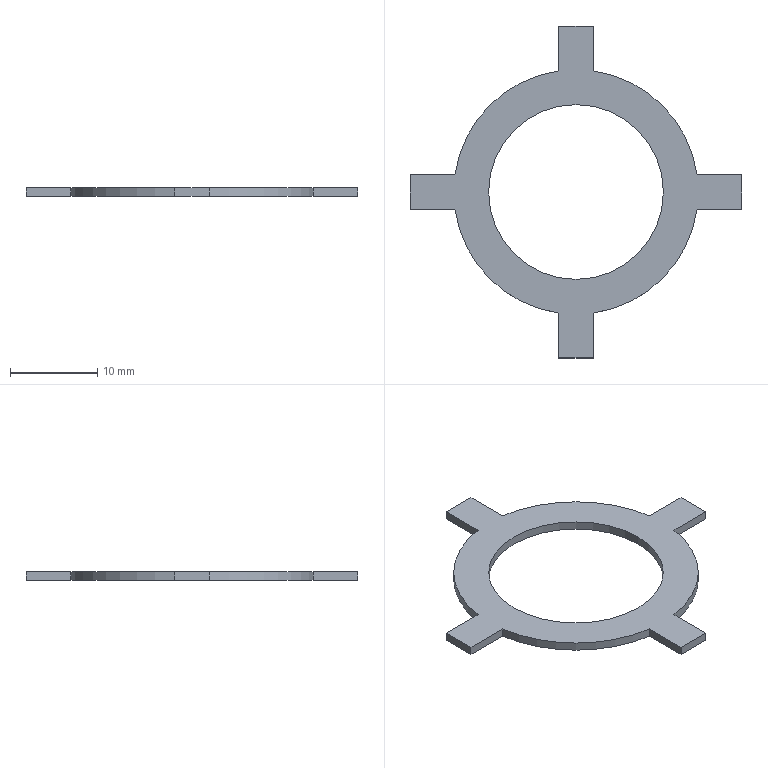Part | STEP file | ZDDQ-M20 | 1 solid | 20 faces | box 38 x 38 x 1 mm | volume 382.357 mm3 | plane 14 | cylinder 6 | commonest cylinder face diameters 28 x4 20 x2
STEP:
#1=CARTESIAN_POINT('',(-19.,2.,0.));
#2=VERTEX_POINT('',#1);
#3=CARTESIAN_POINT('',(-19.,-2.,0.));
#4=VERTEX_POINT('',#3);
#5=CARTESIAN_POINT('',(-19.,0.,0.));
#6=DIRECTION('',(0.,1.,0.));
#7=VECTOR('',#6,1.);
#8=LINE('',#5,#7);
#9=EDGE_CURVE('',#2,#4,#8,.F.);
#10=ORIENTED_EDGE('',*,*,#9,.T.);
#11=CARTESIAN_POINT('',(-19.,-2.,1.));
#12=VERTEX_POINT('',#11);
#13=CARTESIAN_POINT('',(-19.,-2.,0.5));
#14=DIRECTION('',(0.,0.,-1.));
#15=VECTOR('',#14,1.);
#16=LINE('',#13,#15);
#17=EDGE_CURVE('',#12,#4,#16,.T.);
#18=ORIENTED_EDGE('',*,*,#17,.F.);
#19=CARTESIAN_POINT('',(-19.,2.,1.));
#20=VERTEX_POINT('',#19);
#21=CARTESIAN_POINT('',(-19.,0.,1.));
#22=DIRECTION('',(0.,1.,0.));
#23=VECTOR('',#22,1.);
#24=LINE('',#21,#23);
#25=EDGE_CURVE('',#20,#12,#24,.F.);
#26=ORIENTED_EDGE('',*,*,#25,.F.);
#27=CARTESIAN_POINT('',(-19.,2.,0.5));
#28=DIRECTION('',(0.,0.,-1.));
#29=VECTOR('',#28,1.);
#30=LINE('',#27,#29);
#31=EDGE_CURVE('',#20,#2,#30,.T.);
#32=ORIENTED_EDGE('',*,*,#31,.T.);
#33=EDGE_LOOP('',(#10,#18,#26,#32));
#34=FACE_OUTER_BOUND('',#33,.T.);
#35=CARTESIAN_POINT('',(-19.,-2.,1.));
#36=DIRECTION('',(-1.,0.,0.));
#37=DIRECTION('',(0.,1.,0.));
#38=AXIS2_PLACEMENT_3D('',#35,#36,#37);
#39=PLANE('',#38);
#40=ADVANCED_FACE('',(#34),#39,.T.);
#41=CARTESIAN_POINT('',(-13.856,-2.,0.));
#42=VERTEX_POINT('',#41);
#43=CARTESIAN_POINT('',(-13.856,-2.,1.));
#44=VERTEX_POINT('',#43);
#45=CARTESIAN_POINT('',(-13.856,-2.,0.5));
#46=DIRECTION('',(0.,0.,1.));
#47=VECTOR('',#46,1.);
#48=LINE('',#45,#47);
#49=EDGE_CURVE('',#42,#44,#48,.T.);
#50=ORIENTED_EDGE('',*,*,#49,.T.);
#51=CARTESIAN_POINT('',(-16.428,-2.,1.));
#52=DIRECTION('',(1.,0.,0.));
#53=VECTOR('',#52,1.);
#54=LINE('',#51,#53);
#55=EDGE_CURVE('',#12,#44,#54,.T.);
#56=ORIENTED_EDGE('',*,*,#55,.F.);
#57=ORIENTED_EDGE('',*,*,#17,.T.);
#58=CARTESIAN_POINT('',(-16.428,-2.,0.));
#59=DIRECTION('',(1.,0.,0.));
#60=VECTOR('',#59,1.);
#61=LINE('',#58,#60);
#62=EDGE_CURVE('',#4,#42,#61,.T.);
#63=ORIENTED_EDGE('',*,*,#62,.T.);
#64=EDGE_LOOP('',(#50,#56,#57,#63));
#65=FACE_OUTER_BOUND('',#64,.T.);
#66=CARTESIAN_POINT('',(11.858,-2.,1.));
#67=DIRECTION('',(0.,1.,0.));
#68=DIRECTION('',(1.,0.,0.));
#69=AXIS2_PLACEMENT_3D('',#66,#67,#68);
#70=PLANE('',#69);
#71=ADVANCED_FACE('',(#65),#70,.F.);
#72=CARTESIAN_POINT('',(-13.856,2.,0.));
#73=VERTEX_POINT('',#72);
#74=CARTESIAN_POINT('',(-13.856,2.,1.));
#75=VERTEX_POINT('',#74);
#76=CARTESIAN_POINT('',(-13.856,2.,0.5));
#77=DIRECTION('',(0.,0.,1.));
#78=VECTOR('',#77,1.);
#79=LINE('',#76,#78);
#80=EDGE_CURVE('',#73,#75,#79,.T.);
#81=ORIENTED_EDGE('',*,*,#80,.F.);
#82=CARTESIAN_POINT('',(-16.428,2.,0.));
#83=DIRECTION('',(-1.,0.,0.));
#84=VECTOR('',#83,1.);
#85=LINE('',#82,#84);
#86=EDGE_CURVE('',#73,#2,#85,.T.);
#87=ORIENTED_EDGE('',*,*,#86,.T.);
#88=ORIENTED_EDGE('',*,*,#31,.F.);
#89=CARTESIAN_POINT('',(-16.428,2.,1.));
#90=DIRECTION('',(-1.,0.,0.));
#91=VECTOR('',#90,1.);
#92=LINE('',#89,#91);
#93=EDGE_CURVE('',#75,#20,#92,.T.);
#94=ORIENTED_EDGE('',*,*,#93,.F.);
#95=EDGE_LOOP('',(#81,#87,#88,#94));
#96=FACE_OUTER_BOUND('',#95,.T.);
#97=CARTESIAN_POINT('',(19.,2.,1.));
#98=DIRECTION('',(0.,-1.,0.));
#99=DIRECTION('',(-1.,0.,0.));
#100=AXIS2_PLACEMENT_3D('',#97,#98,#99);
#101=PLANE('',#100);
#102=ADVANCED_FACE('',(#96),#101,.F.);
#103=CARTESIAN_POINT('',(-2.,-19.,0.));
#104=VERTEX_POINT('',#103);
#105=CARTESIAN_POINT('',(2.,-19.,0.));
#106=VERTEX_POINT('',#105);
#107=CARTESIAN_POINT('',(0.,-19.,0.));
#108=DIRECTION('',(-1.,0.,0.));
#109=VECTOR('',#108,1.);
#110=LINE('',#107,#109);
#111=EDGE_CURVE('',#104,#106,#110,.F.);
#112=ORIENTED_EDGE('',*,*,#111,.T.);
#113=CARTESIAN_POINT('',(2.,-19.,1.));
#114=VERTEX_POINT('',#113);
#115=CARTESIAN_POINT('',(2.,-19.,0.5));
#116=DIRECTION('',(0.,0.,-1.));
#117=VECTOR('',#116,1.);
#118=LINE('',#115,#117);
#119=EDGE_CURVE('',#114,#106,#118,.T.);
#120=ORIENTED_EDGE('',*,*,#119,.F.);
#121=CARTESIAN_POINT('',(-2.,-19.,1.));
#122=VERTEX_POINT('',#121);
#123=CARTESIAN_POINT('',(0.,-19.,1.));
#124=DIRECTION('',(-1.,0.,0.));
#125=VECTOR('',#124,1.);
#126=LINE('',#123,#125);
#127=EDGE_CURVE('',#122,#114,#126,.F.);
#128=ORIENTED_EDGE('',*,*,#127,.F.);
#129=CARTESIAN_POINT('',(-2.,-19.,0.5));
#130=DIRECTION('',(0.,0.,-1.));
#131=VECTOR('',#130,1.);
#132=LINE('',#129,#131);
#133=EDGE_CURVE('',#122,#104,#132,.T.);
#134=ORIENTED_EDGE('',*,*,#133,.T.);
#135=EDGE_LOOP('',(#112,#120,#128,#134));
#136=FACE_OUTER_BOUND('',#135,.T.);
#137=CARTESIAN_POINT('',(2.,-19.,1.));
#138=DIRECTION('',(0.,-1.,0.));
#139=DIRECTION('',(-1.,0.,0.));
#140=AXIS2_PLACEMENT_3D('',#137,#138,#139);
#141=PLANE('',#140);
#142=ADVANCED_FACE('',(#136),#141,.T.);
#143=CARTESIAN_POINT('',(2.,-13.856,0.));
#144=VERTEX_POINT('',#143);
#145=CARTESIAN_POINT('',(2.,-13.856,1.));
#146=VERTEX_POINT('',#145);
#147=CARTESIAN_POINT('',(2.,-13.856,0.5));
#148=DIRECTION('',(0.,0.,1.));
#149=VECTOR('',#148,1.);
#150=LINE('',#147,#149);
#151=EDGE_CURVE('',#144,#146,#150,.T.);
#152=ORIENTED_EDGE('',*,*,#151,.T.);
#153=CARTESIAN_POINT('',(2.,-16.428,1.));
#154=DIRECTION('',(0.,1.,0.));
#155=VECTOR('',#154,1.);
#156=LINE('',#153,#155);
#157=EDGE_CURVE('',#114,#146,#156,.T.);
#158=ORIENTED_EDGE('',*,*,#157,.F.);
#159=ORIENTED_EDGE('',*,*,#119,.T.);
#160=CARTESIAN_POINT('',(2.,-16.428,0.));
#161=DIRECTION('',(0.,1.,0.));
#162=VECTOR('',#161,1.);
#163=LINE('',#160,#162);
#164=EDGE_CURVE('',#106,#144,#163,.T.);
#165=ORIENTED_EDGE('',*,*,#164,.T.);
#166=EDGE_LOOP('',(#152,#158,#159,#165));
#167=FACE_OUTER_BOUND('',#166,.T.);
#168=CARTESIAN_POINT('',(2.,11.858,1.));
#169=DIRECTION('',(-1.,0.,0.));
#170=DIRECTION('',(0.,1.,0.));
#171=AXIS2_PLACEMENT_3D('',#168,#169,#170);
#172=PLANE('',#171);
#173=ADVANCED_FACE('',(#167),#172,.F.);
#174=CARTESIAN_POINT('',(-2.,-13.856,0.));
#175=VERTEX_POINT('',#174);
#176=CARTESIAN_POINT('',(-2.,-13.856,1.));
#177=VERTEX_POINT('',#176);
#178=CARTESIAN_POINT('',(-2.,-13.856,0.5));
#179=DIRECTION('',(0.,0.,1.));
#180=VECTOR('',#179,1.);
#181=LINE('',#178,#180);
#182=EDGE_CURVE('',#175,#177,#181,.T.);
#183=ORIENTED_EDGE('',*,*,#182,.F.);
#184=CARTESIAN_POINT('',(-2.,-16.428,0.));
#185=DIRECTION('',(0.,-1.,0.));
#186=VECTOR('',#185,1.);
#187=LINE('',#184,#186);
#188=EDGE_CURVE('',#175,#104,#187,.T.);
#189=ORIENTED_EDGE('',*,*,#188,.T.);
#190=ORIENTED_EDGE('',*,*,#133,.F.);
#191=CARTESIAN_POINT('',(-2.,-16.428,1.));
#192=DIRECTION('',(0.,-1.,0.));
#193=VECTOR('',#192,1.);
#194=LINE('',#191,#193);
#195=EDGE_CURVE('',#177,#122,#194,.T.);
#196=ORIENTED_EDGE('',*,*,#195,.F.);
#197=EDGE_LOOP('',(#183,#189,#190,#196));
#198=FACE_OUTER_BOUND('',#197,.T.);
#199=CARTESIAN_POINT('',(-2.,19.,1.));
#200=DIRECTION('',(1.,0.,0.));
#201=DIRECTION('',(0.,-1.,0.));
#202=AXIS2_PLACEMENT_3D('',#199,#200,#201);
#203=PLANE('',#202);
#204=ADVANCED_FACE('',(#198),#203,.F.);
#205=CARTESIAN_POINT('',(19.,-2.,0.));
#206=VERTEX_POINT('',#205);
#207=CARTESIAN_POINT('',(19.,2.,0.));
#208=VERTEX_POINT('',#207);
#209=CARTESIAN_POINT('',(19.,0.,0.));
#210=DIRECTION('',(0.,-1.,0.));
#211=VECTOR('',#210,1.);
#212=LINE('',#209,#211);
#213=EDGE_CURVE('',#206,#208,#212,.F.);
#214=ORIENTED_EDGE('',*,*,#213,.T.);
#215=CARTESIAN_POINT('',(19.,2.,1.));
#216=VERTEX_POINT('',#215);
#217=CARTESIAN_POINT('',(19.,2.,0.5));
#218=DIRECTION('',(0.,0.,-1.));
#219=VECTOR('',#218,1.);
#220=LINE('',#217,#219);
#221=EDGE_CURVE('',#216,#208,#220,.T.);
#222=ORIENTED_EDGE('',*,*,#221,.F.);
#223=CARTESIAN_POINT('',(19.,-2.,1.));
#224=VERTEX_POINT('',#223);
#225=CARTESIAN_POINT('',(19.,0.,1.));
#226=DIRECTION('',(0.,-1.,0.));
#227=VECTOR('',#226,1.);
#228=LINE('',#225,#227);
#229=EDGE_CURVE('',#224,#216,#228,.F.);
#230=ORIENTED_EDGE('',*,*,#229,.F.);
#231=CARTESIAN_POINT('',(19.,-2.,0.5));
#232=DIRECTION('',(0.,0.,-1.));
#233=VECTOR('',#232,1.);
#234=LINE('',#231,#233);
#235=EDGE_CURVE('',#224,#206,#234,.T.);
#236=ORIENTED_EDGE('',*,*,#235,.T.);
#237=EDGE_LOOP('',(#214,#222,#230,#236));
#238=FACE_OUTER_BOUND('',#237,.T.);
#239=CARTESIAN_POINT('',(19.,2.,1.));
#240=DIRECTION('',(1.,0.,0.));
#241=DIRECTION('',(0.,-1.,0.));
#242=AXIS2_PLACEMENT_3D('',#239,#240,#241);
#243=PLANE('',#242);
#244=ADVANCED_FACE('',(#238),#243,.T.);
#245=CARTESIAN_POINT('',(13.856,2.,0.));
#246=VERTEX_POINT('',#245);
#247=CARTESIAN_POINT('',(13.856,2.,1.));
#248=VERTEX_POINT('',#247);
#249=CARTESIAN_POINT('',(13.856,2.,0.5));
#250=DIRECTION('',(0.,0.,1.));
#251=VECTOR('',#250,1.);
#252=LINE('',#249,#251);
#253=EDGE_CURVE('',#246,#248,#252,.T.);
#254=ORIENTED_EDGE('',*,*,#253,.T.);
#255=CARTESIAN_POINT('',(16.428,2.,1.));
#256=DIRECTION('',(-1.,0.,0.));
#257=VECTOR('',#256,1.);
#258=LINE('',#255,#257);
#259=EDGE_CURVE('',#216,#248,#258,.T.);
#260=ORIENTED_EDGE('',*,*,#259,.F.);
#261=ORIENTED_EDGE('',*,*,#221,.T.);
#262=CARTESIAN_POINT('',(16.428,2.,0.));
#263=DIRECTION('',(-1.,0.,0.));
#264=VECTOR('',#263,1.);
#265=LINE('',#262,#264);
#266=EDGE_CURVE('',#208,#246,#265,.T.);
#267=ORIENTED_EDGE('',*,*,#266,.T.);
#268=EDGE_LOOP('',(#254,#260,#261,#267));
#269=FACE_OUTER_BOUND('',#268,.T.);
#270=ADVANCED_FACE('',(#269),#101,.F.);
#271=CARTESIAN_POINT('',(13.856,-2.,0.));
#272=VERTEX_POINT('',#271);
#273=CARTESIAN_POINT('',(13.856,-2.,1.));
#274=VERTEX_POINT('',#273);
#275=CARTESIAN_POINT('',(13.856,-2.,0.5));
#276=DIRECTION('',(0.,0.,1.));
#277=VECTOR('',#276,1.);
#278=LINE('',#275,#277);
#279=EDGE_CURVE('',#272,#274,#278,.T.);
#280=ORIENTED_EDGE('',*,*,#279,.F.);
#281=CARTESIAN_POINT('',(16.428,-2.,0.));
#282=DIRECTION('',(1.,0.,0.));
#283=VECTOR('',#282,1.);
#284=LINE('',#281,#283);
#285=EDGE_CURVE('',#272,#206,#284,.T.);
#286=ORIENTED_EDGE('',*,*,#285,.T.);
#287=ORIENTED_EDGE('',*,*,#235,.F.);
#288=CARTESIAN_POINT('',(16.428,-2.,1.));
#289=DIRECTION('',(1.,0.,0.));
#290=VECTOR('',#289,1.);
#291=LINE('',#288,#290);
#292=EDGE_CURVE('',#274,#224,#291,.T.);
#293=ORIENTED_EDGE('',*,*,#292,.F.);
#294=EDGE_LOOP('',(#280,#286,#287,#293));
#295=FACE_OUTER_BOUND('',#294,.T.);
#296=ADVANCED_FACE('',(#295),#70,.F.);
#297=CARTESIAN_POINT('',(-10.,0.,1.));
#298=VERTEX_POINT('',#297);
#299=CARTESIAN_POINT('',(10.,0.,1.));
#300=VERTEX_POINT('',#299);
#301=CARTESIAN_POINT('',(0.,0.,1.));
#302=DIRECTION('',(0.,0.,1.));
#303=AXIS2_PLACEMENT_3D('',#301,#302,$);
#304=CIRCLE('',#303,10.);
#305=EDGE_CURVE('',#298,#300,#304,.T.);
#306=ORIENTED_EDGE('',*,*,#305,.T.);
#307=CARTESIAN_POINT('',(10.,0.,0.));
#308=VERTEX_POINT('',#307);
#309=CARTESIAN_POINT('',(10.,0.,0.5));
#310=DIRECTION('',(0.,0.,1.));
#311=VECTOR('',#310,1.);
#312=LINE('',#309,#311);
#313=EDGE_CURVE('',#308,#300,#312,.T.);
#314=ORIENTED_EDGE('',*,*,#313,.F.);
#315=CARTESIAN_POINT('',(-10.,0.,0.));
#316=VERTEX_POINT('',#315);
#317=CARTESIAN_POINT('',(0.,0.,0.));
#318=DIRECTION('',(0.,0.,1.));
#319=AXIS2_PLACEMENT_3D('',#317,#318,$);
#320=CIRCLE('',#319,10.);
#321=EDGE_CURVE('',#316,#308,#320,.T.);
#322=ORIENTED_EDGE('',*,*,#321,.F.);
#323=CARTESIAN_POINT('',(-10.,0.,0.5));
#324=DIRECTION('',(0.,0.,1.));
#325=VECTOR('',#324,1.);
#326=LINE('',#323,#325);
#327=EDGE_CURVE('',#316,#298,#326,.T.);
#328=ORIENTED_EDGE('',*,*,#327,.T.);
#329=EDGE_LOOP('',(#306,#314,#322,#328));
#330=FACE_OUTER_BOUND('',#329,.T.);
#331=CARTESIAN_POINT('',(0.,0.,0.5));
#332=DIRECTION('',(0.,0.,1.));
#333=DIRECTION('',(1.,0.,0.));
#334=AXIS2_PLACEMENT_3D('',#331,#332,#333);
#335=CYLINDRICAL_SURFACE('',#334,10.);
#336=ADVANCED_FACE('',(#330),#335,.F.);
#337=CARTESIAN_POINT('',(0.,0.,1.));
#338=DIRECTION('',(0.,0.,1.));
#339=AXIS2_PLACEMENT_3D('',#337,#338,$);
#340=CIRCLE('',#339,10.);
#341=EDGE_CURVE('',#300,#298,#340,.T.);
#342=ORIENTED_EDGE('',*,*,#341,.T.);
#343=ORIENTED_EDGE('',*,*,#327,.F.);
#344=CARTESIAN_POINT('',(0.,0.,0.));
#345=DIRECTION('',(0.,0.,1.));
#346=AXIS2_PLACEMENT_3D('',#344,#345,$);
#347=CIRCLE('',#346,10.);
#348=EDGE_CURVE('',#308,#316,#347,.T.);
#349=ORIENTED_EDGE('',*,*,#348,.F.);
#350=ORIENTED_EDGE('',*,*,#313,.T.);
#351=EDGE_LOOP('',(#342,#343,#349,#350));
#352=FACE_OUTER_BOUND('',#351,.T.);
#353=ADVANCED_FACE('',(#352),#335,.F.);
#354=CARTESIAN_POINT('',(-2.,13.856,0.));
#355=VERTEX_POINT('',#354);
#356=CARTESIAN_POINT('',(-2.,13.856,1.));
#357=VERTEX_POINT('',#356);
#358=CARTESIAN_POINT('',(-2.,13.856,0.5));
#359=DIRECTION('',(0.,0.,1.));
#360=VECTOR('',#359,1.);
#361=LINE('',#358,#360);
#362=EDGE_CURVE('',#355,#357,#361,.T.);
#363=ORIENTED_EDGE('',*,*,#362,.F.);
#364=CARTESIAN_POINT('',(0.,0.,0.));
#365=DIRECTION('',(0.,0.,1.));
#366=AXIS2_PLACEMENT_3D('',#364,#365,$);
#367=CIRCLE('',#366,14.);
#368=EDGE_CURVE('',#355,#73,#367,.T.);
#369=ORIENTED_EDGE('',*,*,#368,.T.);
#370=ORIENTED_EDGE('',*,*,#80,.T.);
#371=CARTESIAN_POINT('',(0.,0.,1.));
#372=DIRECTION('',(0.,0.,1.));
#373=AXIS2_PLACEMENT_3D('',#371,#372,$);
#374=CIRCLE('',#373,14.);
#375=EDGE_CURVE('',#357,#75,#374,.T.);
#376=ORIENTED_EDGE('',*,*,#375,.F.);
#377=EDGE_LOOP('',(#363,#369,#370,#376));
#378=FACE_OUTER_BOUND('',#377,.T.);
#379=CARTESIAN_POINT('',(0.,0.,0.5));
#380=DIRECTION('',(0.,0.,1.));
#381=DIRECTION('',(1.,0.,0.));
#382=AXIS2_PLACEMENT_3D('',#379,#380,#381);
#383=CYLINDRICAL_SURFACE('',#382,14.);
#384=ADVANCED_FACE('',(#378),#383,.T.);
#385=ORIENTED_EDGE('',*,*,#182,.T.);
#386=CARTESIAN_POINT('',(0.,0.,1.));
#387=DIRECTION('',(0.,0.,1.));
#388=AXIS2_PLACEMENT_3D('',#386,#387,$);
#389=CIRCLE('',#388,14.);
#390=EDGE_CURVE('',#44,#177,#389,.T.);
#391=ORIENTED_EDGE('',*,*,#390,.F.);
#392=ORIENTED_EDGE('',*,*,#49,.F.);
#393=CARTESIAN_POINT('',(0.,0.,0.));
#394=DIRECTION('',(0.,0.,1.));
#395=AXIS2_PLACEMENT_3D('',#393,#394,$);
#396=CIRCLE('',#395,14.);
#397=EDGE_CURVE('',#42,#175,#396,.T.);
#398=ORIENTED_EDGE('',*,*,#397,.T.);
#399=EDGE_LOOP('',(#385,#391,#392,#398));
#400=FACE_OUTER_BOUND('',#399,.T.);
#401=ADVANCED_FACE('',(#400),#383,.T.);
#402=ORIENTED_EDGE('',*,*,#151,.F.);
#403=CARTESIAN_POINT('',(0.,0.,0.));
#404=DIRECTION('',(0.,0.,1.));
#405=AXIS2_PLACEMENT_3D('',#403,#404,$);
#406=CIRCLE('',#405,14.);
#407=EDGE_CURVE('',#144,#272,#406,.T.);
#408=ORIENTED_EDGE('',*,*,#407,.T.);
#409=ORIENTED_EDGE('',*,*,#279,.T.);
#410=CARTESIAN_POINT('',(0.,0.,1.));
#411=DIRECTION('',(0.,0.,1.));
#412=AXIS2_PLACEMENT_3D('',#410,#411,$);
#413=CIRCLE('',#412,14.);
#414=EDGE_CURVE('',#146,#274,#413,.T.);
#415=ORIENTED_EDGE('',*,*,#414,.F.);
#416=EDGE_LOOP('',(#402,#408,#409,#415));
#417=FACE_OUTER_BOUND('',#416,.T.);
#418=ADVANCED_FACE('',(#417),#383,.T.);
#419=CARTESIAN_POINT('',(2.,13.856,0.));
#420=VERTEX_POINT('',#419);
#421=CARTESIAN_POINT('',(2.,13.856,1.));
#422=VERTEX_POINT('',#421);
#423=CARTESIAN_POINT('',(2.,13.856,0.5));
#424=DIRECTION('',(0.,0.,1.));
#425=VECTOR('',#424,1.);
#426=LINE('',#423,#425);
#427=EDGE_CURVE('',#420,#422,#426,.T.);
#428=ORIENTED_EDGE('',*,*,#427,.T.);
#429=CARTESIAN_POINT('',(0.,0.,1.));
#430=DIRECTION('',(0.,0.,1.));
#431=AXIS2_PLACEMENT_3D('',#429,#430,$);
#432=CIRCLE('',#431,14.);
#433=EDGE_CURVE('',#248,#422,#432,.T.);
#434=ORIENTED_EDGE('',*,*,#433,.F.);
#435=ORIENTED_EDGE('',*,*,#253,.F.);
#436=CARTESIAN_POINT('',(0.,0.,0.));
#437=DIRECTION('',(0.,0.,1.));
#438=AXIS2_PLACEMENT_3D('',#436,#437,$);
#439=CIRCLE('',#438,14.);
#440=EDGE_CURVE('',#246,#420,#439,.T.);
#441=ORIENTED_EDGE('',*,*,#440,.T.);
#442=EDGE_LOOP('',(#428,#434,#435,#441));
#443=FACE_OUTER_BOUND('',#442,.T.);
#444=ADVANCED_FACE('',(#443),#383,.T.);
#445=CARTESIAN_POINT('',(2.,19.,0.));
#446=VERTEX_POINT('',#445);
#447=CARTESIAN_POINT('',(-2.,19.,0.));
#448=VERTEX_POINT('',#447);
#449=CARTESIAN_POINT('',(0.,19.,0.));
#450=DIRECTION('',(1.,0.,0.));
#451=VECTOR('',#450,1.);
#452=LINE('',#449,#451);
#453=EDGE_CURVE('',#446,#448,#452,.F.);
#454=ORIENTED_EDGE('',*,*,#453,.T.);
#455=CARTESIAN_POINT('',(-2.,19.,1.));
#456=VERTEX_POINT('',#455);
#457=CARTESIAN_POINT('',(-2.,19.,0.5));
#458=DIRECTION('',(0.,0.,-1.));
#459=VECTOR('',#458,1.);
#460=LINE('',#457,#459);
#461=EDGE_CURVE('',#456,#448,#460,.T.);
#462=ORIENTED_EDGE('',*,*,#461,.F.);
#463=CARTESIAN_POINT('',(2.,19.,1.));
#464=VERTEX_POINT('',#463);
#465=CARTESIAN_POINT('',(0.,19.,1.));
#466=DIRECTION('',(1.,0.,0.));
#467=VECTOR('',#466,1.);
#468=LINE('',#465,#467);
#469=EDGE_CURVE('',#464,#456,#468,.F.);
#470=ORIENTED_EDGE('',*,*,#469,.F.);
#471=CARTESIAN_POINT('',(2.,19.,0.5));
#472=DIRECTION('',(0.,0.,-1.));
#473=VECTOR('',#472,1.);
#474=LINE('',#471,#473);
#475=EDGE_CURVE('',#464,#446,#474,.T.);
#476=ORIENTED_EDGE('',*,*,#475,.T.);
#477=EDGE_LOOP('',(#454,#462,#470,#476));
#478=FACE_OUTER_BOUND('',#477,.T.);
#479=CARTESIAN_POINT('',(-2.,19.,1.));
#480=DIRECTION('',(0.,1.,0.));
#481=DIRECTION('',(1.,0.,0.));
#482=AXIS2_PLACEMENT_3D('',#479,#480,#481);
#483=PLANE('',#482);
#484=ADVANCED_FACE('',(#478),#483,.T.);
#485=ORIENTED_EDGE('',*,*,#362,.T.);
#486=CARTESIAN_POINT('',(-2.,16.428,1.));
#487=DIRECTION('',(0.,-1.,0.));
#488=VECTOR('',#487,1.);
#489=LINE('',#486,#488);
#490=EDGE_CURVE('',#456,#357,#489,.T.);
#491=ORIENTED_EDGE('',*,*,#490,.F.);
#492=ORIENTED_EDGE('',*,*,#461,.T.);
#493=CARTESIAN_POINT('',(-2.,16.428,0.));
#494=DIRECTION('',(0.,-1.,0.));
#495=VECTOR('',#494,1.);
#496=LINE('',#493,#495);
#497=EDGE_CURVE('',#448,#355,#496,.T.);
#498=ORIENTED_EDGE('',*,*,#497,.T.);
#499=EDGE_LOOP('',(#485,#491,#492,#498));
#500=FACE_OUTER_BOUND('',#499,.T.);
#501=ADVANCED_FACE('',(#500),#203,.F.);
#502=ORIENTED_EDGE('',*,*,#427,.F.);
#503=CARTESIAN_POINT('',(2.,16.428,0.));
#504=DIRECTION('',(0.,1.,0.));
#505=VECTOR('',#504,1.);
#506=LINE('',#503,#505);
#507=EDGE_CURVE('',#420,#446,#506,.T.);
#508=ORIENTED_EDGE('',*,*,#507,.T.);
#509=ORIENTED_EDGE('',*,*,#475,.F.);
#510=CARTESIAN_POINT('',(2.,16.428,1.));
#511=DIRECTION('',(0.,1.,0.));
#512=VECTOR('',#511,1.);
#513=LINE('',#510,#512);
#514=EDGE_CURVE('',#422,#464,#513,.T.);
#515=ORIENTED_EDGE('',*,*,#514,.F.);
#516=EDGE_LOOP('',(#502,#508,#509,#515));
#517=FACE_OUTER_BOUND('',#516,.T.);
#518=ADVANCED_FACE('',(#517),#172,.F.);
#519=ORIENTED_EDGE('',*,*,#514,.T.);
#520=ORIENTED_EDGE('',*,*,#469,.T.);
#521=ORIENTED_EDGE('',*,*,#490,.T.);
#522=ORIENTED_EDGE('',*,*,#375,.T.);
#523=ORIENTED_EDGE('',*,*,#93,.T.);
#524=ORIENTED_EDGE('',*,*,#25,.T.);
#525=ORIENTED_EDGE('',*,*,#55,.T.);
#526=ORIENTED_EDGE('',*,*,#390,.T.);
#527=ORIENTED_EDGE('',*,*,#195,.T.);
#528=ORIENTED_EDGE('',*,*,#127,.T.);
#529=ORIENTED_EDGE('',*,*,#157,.T.);
#530=ORIENTED_EDGE('',*,*,#414,.T.);
#531=ORIENTED_EDGE('',*,*,#292,.T.);
#532=ORIENTED_EDGE('',*,*,#229,.T.);
#533=ORIENTED_EDGE('',*,*,#259,.T.);
#534=ORIENTED_EDGE('',*,*,#433,.T.);
#535=EDGE_LOOP('',(#519,#520,#521,#522,#523,#524,#525,#526,#527,#528,#529,#530,#531,#532,#533,#534));
#536=FACE_OUTER_BOUND('',#535,.T.);
#537=ORIENTED_EDGE('',*,*,#341,.F.);
#538=ORIENTED_EDGE('',*,*,#305,.F.);
#539=EDGE_LOOP('',(#537,#538));
#540=FACE_BOUND('',#539,.T.);
#541=CARTESIAN_POINT('',(0.,0.,1.));
#542=DIRECTION('',(0.,0.,1.));
#543=DIRECTION('',(1.,0.,0.));
#544=AXIS2_PLACEMENT_3D('',#541,#542,#543);
#545=PLANE('',#544);
#546=ADVANCED_FACE('',(#536,#540),#545,.T.);
#547=ORIENTED_EDGE('',*,*,#440,.F.);
#548=ORIENTED_EDGE('',*,*,#266,.F.);
#549=ORIENTED_EDGE('',*,*,#213,.F.);
#550=ORIENTED_EDGE('',*,*,#285,.F.);
#551=ORIENTED_EDGE('',*,*,#407,.F.);
#552=ORIENTED_EDGE('',*,*,#164,.F.);
#553=ORIENTED_EDGE('',*,*,#111,.F.);
#554=ORIENTED_EDGE('',*,*,#188,.F.);
#555=ORIENTED_EDGE('',*,*,#397,.F.);
#556=ORIENTED_EDGE('',*,*,#62,.F.);
#557=ORIENTED_EDGE('',*,*,#9,.F.);
#558=ORIENTED_EDGE('',*,*,#86,.F.);
#559=ORIENTED_EDGE('',*,*,#368,.F.);
#560=ORIENTED_EDGE('',*,*,#497,.F.);
#561=ORIENTED_EDGE('',*,*,#453,.F.);
#562=ORIENTED_EDGE('',*,*,#507,.F.);
#563=EDGE_LOOP('',(#547,#548,#549,#550,#551,#552,#553,#554,#555,#556,#557,#558,#559,#560,#561,#562));
#564=FACE_OUTER_BOUND('',#563,.T.);
#565=ORIENTED_EDGE('',*,*,#321,.T.);
#566=ORIENTED_EDGE('',*,*,#348,.T.);
#567=EDGE_LOOP('',(#565,#566));
#568=FACE_BOUND('',#567,.T.);
#569=CARTESIAN_POINT('',(0.,0.,0.));
#570=DIRECTION('',(0.,0.,1.));
#571=DIRECTION('',(1.,0.,0.));
#572=AXIS2_PLACEMENT_3D('',#569,#570,#571);
#573=PLANE('',#572);
#574=ADVANCED_FACE('',(#564,#568),#573,.F.);
#575=CLOSED_SHELL('',(#40,#71,#102,#142,#173,#204,#244,#270,#296,#336,#353,#384,#401,#418,#444,#484,#501,#518,#546,#574));
#576=MANIFOLD_SOLID_BREP('',#575);
#577=(LENGTH_UNIT()NAMED_UNIT(*)SI_UNIT(.MILLI.,.METRE.));
#578=UNCERTAINTY_MEASURE_WITH_UNIT(LENGTH_MEASURE(0.005),#577,'','');
#579=(NAMED_UNIT(*)PLANE_ANGLE_UNIT()SI_UNIT($,.RADIAN.));
#580=(NAMED_UNIT(*)SI_UNIT($,.STERADIAN.)SOLID_ANGLE_UNIT());
#581=(GEOMETRIC_REPRESENTATION_CONTEXT(3)GLOBAL_UNCERTAINTY_ASSIGNED_CONTEXT((#578))GLOBAL_UNIT_ASSIGNED_CONTEXT((#577,#579,#580))REPRESENTATION_CONTEXT('',''));
#582=ADVANCED_BREP_SHAPE_REPRESENTATION('',(#576),#581);